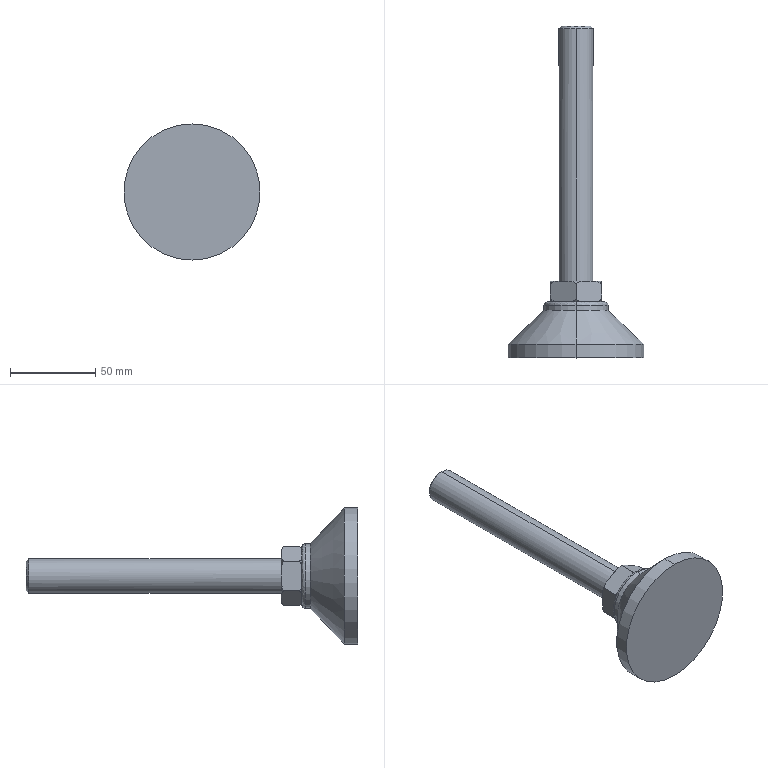Part | SolidWorks | features BaseBody 1 | 1 solid | 36 faces | box 80 x 195 x 80 mm | volume 159151 mm3 | spline 16 | plane 10 | cylinder 6 | cone 4 | commonest cylinder face diameters 20 x2 38 x2 80 x2